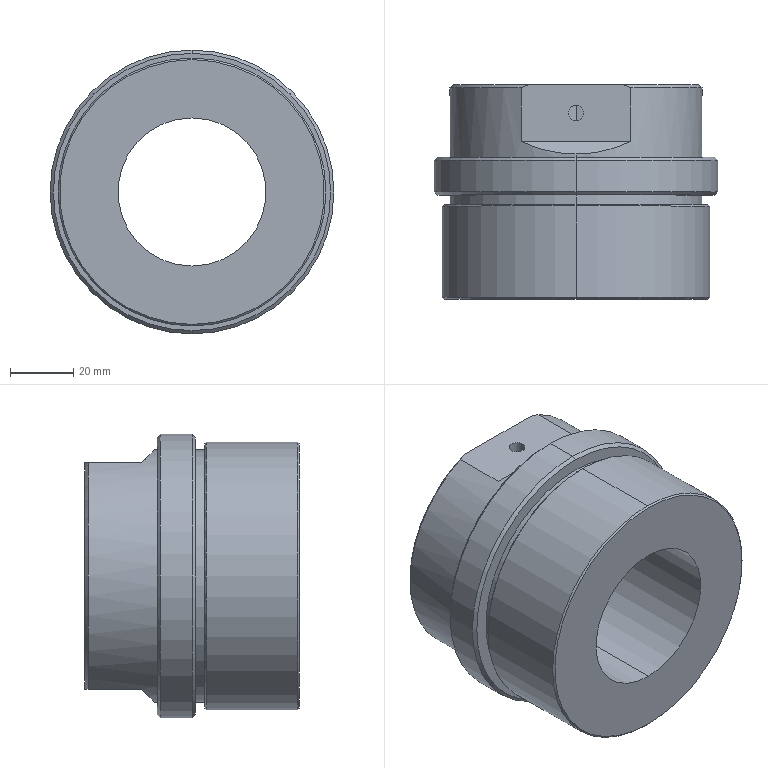Part | SolidWorks | features ICE 14, Chamfer 4, HoleWzd 2, Extrusion 1 | 1 solid | 31 faces | box 90 x 68 x 90 mm | volume 254922 mm3 | cylinder 12 | cone 10 | plane 9 | commonest cylinder face diameters 80 x4 5 x2 47 x2 85 x2 90 x2
STEP:
#1=CARTESIAN_POINT('',(-2.5,21.,23.367));
#2=VERTEX_POINT('',#1);
#3=CARTESIAN_POINT('',(0.,18.5,23.5));
#4=VERTEX_POINT('',#3);
#5=CARTESIAN_POINT('',(-2.5,21.,23.367));
#6=CARTESIAN_POINT('',(-2.5,20.835,23.367));
#7=CARTESIAN_POINT('',(-2.484,20.672,23.368));
#8=CARTESIAN_POINT('',(-2.42,20.353,23.375));
#9=CARTESIAN_POINT('',(-2.372,20.194,23.38));
#10=CARTESIAN_POINT('',(-2.247,19.892,23.392));
#11=CARTESIAN_POINT('',(-2.17,19.748,23.4));
#12=CARTESIAN_POINT('',(-1.989,19.477,23.416));
#13=CARTESIAN_POINT('',(-1.883,19.348,23.425));
#14=CARTESIAN_POINT('',(-1.653,19.118,23.442));
#15=CARTESIAN_POINT('',(-1.528,19.014,23.451));
#16=CARTESIAN_POINT('',(-1.255,18.831,23.467));
#17=CARTESIAN_POINT('',(-1.109,18.754,23.474));
#18=CARTESIAN_POINT('',(-0.6586,18.566,23.493));
#19=CARTESIAN_POINT('',(-0.3304,18.5,23.5));
#20=CARTESIAN_POINT('',(0.,18.5,23.5));
#21=B_SPLINE_CURVE_WITH_KNOTS('',3,(#5,#6,#7,#8,#9,#10,#11,#12,#13,#14,#15,#16,#17,#18,#19,#20),.UNSPECIFIED.,.F.,.F.,(4,2,2,2,2,2,2,4),(0.01173,0.01222,0.01271,0.0132,0.01369,0.01418,0.01466,0.01564),.UNSPECIFIED.);
#22=EDGE_CURVE('',#2,#4,#21,.T.);
#23=ORIENTED_EDGE('',*,*,#22,.F.);
#24=CARTESIAN_POINT('',(-2.5,21.,36.));
#25=VERTEX_POINT('',#24);
#26=CARTESIAN_POINT('',(-2.5,21.,36.));
#27=DIRECTION('',(0.,0.,1.));
#28=VECTOR('',#27,1000.);
#29=LINE('',#26,#28);
#30=EDGE_CURVE('',#2,#25,#29,.T.);
#31=ORIENTED_EDGE('',*,*,#30,.T.);
#32=CARTESIAN_POINT('',(2.5,21.,36.));
#33=VERTEX_POINT('',#32);
#34=CARTESIAN_POINT('',(0.,21.,36.));
#35=DIRECTION('',(0.,0.,1.));
#36=DIRECTION('',(1.,0.,0.));
#37=AXIS2_PLACEMENT_3D('',#34,#35,#36);
#38=CIRCLE('',#37,2.5);
#39=EDGE_CURVE('',#25,#33,#38,.T.);
#40=ORIENTED_EDGE('',*,*,#39,.T.);
#41=CARTESIAN_POINT('',(2.5,21.,23.367));
#42=VERTEX_POINT('',#41);
#43=CARTESIAN_POINT('',(2.5,21.,36.));
#44=DIRECTION('',(0.,0.,1.));
#45=VECTOR('',#44,1000.);
#46=LINE('',#43,#45);
#47=EDGE_CURVE('',#42,#33,#46,.T.);
#48=ORIENTED_EDGE('',*,*,#47,.F.);
#49=CARTESIAN_POINT('',(0.,18.5,23.5));
#50=CARTESIAN_POINT('',(0.1653,18.5,23.5));
#51=CARTESIAN_POINT('',(0.3279,18.516,23.498));
#52=CARTESIAN_POINT('',(0.6477,18.58,23.492));
#53=CARTESIAN_POINT('',(0.8066,18.628,23.487));
#54=CARTESIAN_POINT('',(1.109,18.754,23.474));
#55=CARTESIAN_POINT('',(1.253,18.83,23.467));
#56=CARTESIAN_POINT('',(1.525,19.012,23.451));
#57=CARTESIAN_POINT('',(1.653,19.118,23.442));
#58=CARTESIAN_POINT('',(1.884,19.348,23.425));
#59=CARTESIAN_POINT('',(1.987,19.474,23.416));
#60=CARTESIAN_POINT('',(2.17,19.747,23.4));
#61=CARTESIAN_POINT('',(2.247,19.893,23.392));
#62=CARTESIAN_POINT('',(2.372,20.194,23.38));
#63=CARTESIAN_POINT('',(2.42,20.352,23.375));
#64=CARTESIAN_POINT('',(2.484,20.674,23.368));
#65=CARTESIAN_POINT('',(2.5,20.837,23.367));
#66=CARTESIAN_POINT('',(2.5,21.,23.367));
#67=B_SPLINE_CURVE_WITH_KNOTS('',3,(#49,#50,#51,#52,#53,#54,#55,#56,#57,#58,#59,#60,#61,#62,#63,#64,#65,#66),.UNSPECIFIED.,.F.,.F.,(4,2,2,2,2,2,2,2,4),(0.,0.000489,0.0009779,0.001467,0.001956,0.002445,0.002934,0.003423,0.003912),.UNSPECIFIED.);
#68=EDGE_CURVE('',#4,#42,#67,.T.);
#69=ORIENTED_EDGE('',*,*,#68,.F.);
#70=EDGE_LOOP('',(#23,#31,#40,#48,#69));
#71=FACE_OUTER_BOUND('',#70,.T.);
#72=CARTESIAN_POINT('',(0.,21.,36.));
#73=DIRECTION('',(0.,0.,1.));
#74=DIRECTION('',(1.,0.,0.));
#75=AXIS2_PLACEMENT_3D('',#72,#73,#74);
#76=CYLINDRICAL_SURFACE('',#75,2.5);
#77=ADVANCED_FACE('',(#71),#76,.F.);
#78=CARTESIAN_POINT('',(0.,-8.,42.));
#79=VERTEX_POINT('',#78);
#80=CARTESIAN_POINT('',(0.,-8.,-42.));
#81=VERTEX_POINT('',#80);
#82=CARTESIAN_POINT('',(0.,-8.,0.));
#83=DIRECTION('',(0.,1.,0.));
#84=DIRECTION('',(0.,0.,-1.));
#85=AXIS2_PLACEMENT_3D('',#82,#83,#84);
#86=CIRCLE('',#85,42.);
#87=EDGE_CURVE('',#79,#81,#86,.T.);
#88=ORIENTED_EDGE('',*,*,#87,.F.);
#89=CARTESIAN_POINT('',(0.,-8.5,42.5));
#90=VERTEX_POINT('',#89);
#91=CARTESIAN_POINT('',(0.,-8.5,42.5));
#92=DIRECTION('',(0.,-0.7071,0.7071));
#93=VECTOR('',#92,1000.);
#94=LINE('',#91,#93);
#95=EDGE_CURVE('',#79,#90,#94,.T.);
#96=ORIENTED_EDGE('',*,*,#95,.T.);
#97=CARTESIAN_POINT('',(0.,-8.5,-42.5));
#98=VERTEX_POINT('',#97);
#99=CARTESIAN_POINT('',(0.,-8.5,0.));
#100=DIRECTION('',(0.,-1.,0.));
#101=DIRECTION('',(0.,0.,-1.));
#102=AXIS2_PLACEMENT_3D('',#99,#100,#101);
#103=CIRCLE('',#102,42.5);
#104=EDGE_CURVE('',#98,#90,#103,.T.);
#105=ORIENTED_EDGE('',*,*,#104,.F.);
#106=CARTESIAN_POINT('',(0.,-8.5,-42.5));
#107=DIRECTION('',(0.,-0.7071,-0.7071));
#108=VECTOR('',#107,1000.);
#109=LINE('',#106,#108);
#110=EDGE_CURVE('',#81,#98,#109,.T.);
#111=ORIENTED_EDGE('',*,*,#110,.F.);
#112=EDGE_LOOP('',(#88,#96,#105,#111));
#113=FACE_OUTER_BOUND('',#112,.T.);
#114=CARTESIAN_POINT('',(0.,-8.5,0.));
#115=DIRECTION('',(0.,-1.,0.));
#116=DIRECTION('',(0.,0.,-1.));
#117=AXIS2_PLACEMENT_3D('',#114,#115,#116);
#118=CONICAL_SURFACE('',#117,42.5,0.7854);
#119=ADVANCED_FACE('',(#113),#118,.T.);
#120=CARTESIAN_POINT('',(0.,-38.,-42.));
#121=VERTEX_POINT('',#120);
#122=CARTESIAN_POINT('',(0.,-38.,42.));
#123=VERTEX_POINT('',#122);
#124=CARTESIAN_POINT('',(0.,-38.,0.));
#125=DIRECTION('',(0.,-1.,0.));
#126=DIRECTION('',(0.,0.,-1.));
#127=AXIS2_PLACEMENT_3D('',#124,#125,#126);
#128=CIRCLE('',#127,42.);
#129=EDGE_CURVE('',#121,#123,#128,.T.);
#130=ORIENTED_EDGE('',*,*,#129,.F.);
#131=CARTESIAN_POINT('',(0.,-37.5,-42.5));
#132=VERTEX_POINT('',#131);
#133=CARTESIAN_POINT('',(0.,-38.,-42.));
#134=DIRECTION('',(0.,0.7071,-0.7071));
#135=VECTOR('',#134,1000.);
#136=LINE('',#133,#135);
#137=EDGE_CURVE('',#121,#132,#136,.T.);
#138=ORIENTED_EDGE('',*,*,#137,.T.);
#139=CARTESIAN_POINT('',(0.,-37.5,42.5));
#140=VERTEX_POINT('',#139);
#141=CARTESIAN_POINT('',(0.,-37.5,0.));
#142=DIRECTION('',(0.,1.,0.));
#143=DIRECTION('',(0.,0.,-1.));
#144=AXIS2_PLACEMENT_3D('',#141,#142,#143);
#145=CIRCLE('',#144,42.5);
#146=EDGE_CURVE('',#140,#132,#145,.T.);
#147=ORIENTED_EDGE('',*,*,#146,.F.);
#148=CARTESIAN_POINT('',(0.,-38.,42.));
#149=DIRECTION('',(0.,0.7071,0.7071));
#150=VECTOR('',#149,1000.);
#151=LINE('',#148,#150);
#152=EDGE_CURVE('',#123,#140,#151,.T.);
#153=ORIENTED_EDGE('',*,*,#152,.F.);
#154=EDGE_LOOP('',(#130,#138,#147,#153));
#155=FACE_OUTER_BOUND('',#154,.T.);
#156=CARTESIAN_POINT('',(0.,-38.,0.));
#157=DIRECTION('',(0.,1.,0.));
#158=DIRECTION('',(0.,0.,1.));
#159=AXIS2_PLACEMENT_3D('',#156,#157,#158);
#160=CONICAL_SURFACE('',#159,42.,0.7854);
#161=ADVANCED_FACE('',(#155),#160,.T.);
#162=CARTESIAN_POINT('',(0.,-8.,-40.));
#163=VERTEX_POINT('',#162);
#164=CARTESIAN_POINT('',(0.,-8.,40.));
#165=VERTEX_POINT('',#164);
#166=CARTESIAN_POINT('',(0.,-8.,0.));
#167=DIRECTION('',(0.,-1.,0.));
#168=DIRECTION('',(0.,0.,-1.));
#169=AXIS2_PLACEMENT_3D('',#166,#167,#168);
#170=CIRCLE('',#169,40.);
#171=EDGE_CURVE('',#163,#165,#170,.T.);
#172=ORIENTED_EDGE('',*,*,#171,.F.);
#173=CARTESIAN_POINT('',(0.,-5.,-40.));
#174=VERTEX_POINT('',#173);
#175=CARTESIAN_POINT('',(0.,-8.,-40.));
#176=DIRECTION('',(0.,1.,0.));
#177=VECTOR('',#176,1000.);
#178=LINE('',#175,#177);
#179=EDGE_CURVE('',#163,#174,#178,.T.);
#180=ORIENTED_EDGE('',*,*,#179,.T.);
#181=CARTESIAN_POINT('',(0.,-5.,40.));
#182=VERTEX_POINT('',#181);
#183=CARTESIAN_POINT('',(0.,-5.,0.));
#184=DIRECTION('',(0.,-1.,0.));
#185=DIRECTION('',(0.,0.,-1.));
#186=AXIS2_PLACEMENT_3D('',#183,#184,#185);
#187=CIRCLE('',#186,40.);
#188=EDGE_CURVE('',#174,#182,#187,.T.);
#189=ORIENTED_EDGE('',*,*,#188,.T.);
#190=CARTESIAN_POINT('',(0.,-8.,40.));
#191=DIRECTION('',(0.,1.,0.));
#192=VECTOR('',#191,1000.);
#193=LINE('',#190,#192);
#194=EDGE_CURVE('',#165,#182,#193,.T.);
#195=ORIENTED_EDGE('',*,*,#194,.F.);
#196=EDGE_LOOP('',(#172,#180,#189,#195));
#197=FACE_OUTER_BOUND('',#196,.T.);
#198=CARTESIAN_POINT('',(0.,-8.,0.));
#199=DIRECTION('',(0.,1.,0.));
#200=DIRECTION('',(0.,0.,1.));
#201=AXIS2_PLACEMENT_3D('',#198,#199,#200);
#202=CYLINDRICAL_SURFACE('',#201,40.);
#203=ADVANCED_FACE('',(#197),#202,.T.);
#204=ORIENTED_EDGE('',*,*,#146,.T.);
#205=CARTESIAN_POINT('',(0.,-38.,-42.5));
#206=DIRECTION('',(0.,1.,0.));
#207=VECTOR('',#206,1000.);
#208=LINE('',#205,#207);
#209=EDGE_CURVE('',#132,#98,#208,.T.);
#210=ORIENTED_EDGE('',*,*,#209,.T.);
#211=ORIENTED_EDGE('',*,*,#104,.T.);
#212=CARTESIAN_POINT('',(0.,-38.,42.5));
#213=DIRECTION('',(0.,1.,0.));
#214=VECTOR('',#213,1000.);
#215=LINE('',#212,#214);
#216=EDGE_CURVE('',#140,#90,#215,.T.);
#217=ORIENTED_EDGE('',*,*,#216,.F.);
#218=EDGE_LOOP('',(#204,#210,#211,#217));
#219=FACE_OUTER_BOUND('',#218,.T.);
#220=CARTESIAN_POINT('',(0.,-38.,0.));
#221=DIRECTION('',(0.,1.,0.));
#222=DIRECTION('',(0.,0.,1.));
#223=AXIS2_PLACEMENT_3D('',#220,#221,#222);
#224=CYLINDRICAL_SURFACE('',#223,42.5);
#225=ADVANCED_FACE('',(#219),#224,.T.);
#226=CARTESIAN_POINT('',(0.,-38.,-23.5));
#227=VERTEX_POINT('',#226);
#228=CARTESIAN_POINT('',(0.,-38.,23.5));
#229=VERTEX_POINT('',#228);
#230=CARTESIAN_POINT('',(0.,-38.,0.));
#231=DIRECTION('',(0.,1.,0.));
#232=DIRECTION('',(0.,0.,1.));
#233=AXIS2_PLACEMENT_3D('',#230,#231,#232);
#234=CIRCLE('',#233,23.5);
#235=EDGE_CURVE('',#227,#229,#234,.T.);
#236=ORIENTED_EDGE('',*,*,#235,.F.);
#237=CARTESIAN_POINT('',(0.,30.,-23.5));
#238=VERTEX_POINT('',#237);
#239=CARTESIAN_POINT('',(0.,30.,-23.5));
#240=DIRECTION('',(0.,1.,0.));
#241=VECTOR('',#240,1000.);
#242=LINE('',#239,#241);
#243=EDGE_CURVE('',#227,#238,#242,.T.);
#244=ORIENTED_EDGE('',*,*,#243,.T.);
#245=CARTESIAN_POINT('',(0.,30.,23.5));
#246=VERTEX_POINT('',#245);
#247=CARTESIAN_POINT('',(0.,30.,0.));
#248=DIRECTION('',(0.,1.,0.));
#249=DIRECTION('',(0.,0.,1.));
#250=AXIS2_PLACEMENT_3D('',#247,#248,#249);
#251=CIRCLE('',#250,23.5);
#252=EDGE_CURVE('',#238,#246,#251,.T.);
#253=ORIENTED_EDGE('',*,*,#252,.T.);
#254=CARTESIAN_POINT('',(0.,23.5,23.5));
#255=VERTEX_POINT('',#254);
#256=CARTESIAN_POINT('',(0.,30.,23.5));
#257=DIRECTION('',(0.,1.,0.));
#258=VECTOR('',#257,1000.);
#259=LINE('',#256,#258);
#260=EDGE_CURVE('',#255,#246,#259,.T.);
#261=ORIENTED_EDGE('',*,*,#260,.F.);
#262=CARTESIAN_POINT('',(0.,23.5,23.5));
#263=CARTESIAN_POINT('',(-0.1633,23.5,23.5));
#264=CARTESIAN_POINT('',(-0.3256,23.484,23.498));
#265=CARTESIAN_POINT('',(-0.6484,23.42,23.492));
#266=CARTESIAN_POINT('',(-0.8062,23.372,23.487));
#267=CARTESIAN_POINT('',(-1.107,23.247,23.474));
#268=CARTESIAN_POINT('',(-1.253,23.17,23.467));
#269=CARTESIAN_POINT('',(-1.526,22.987,23.451));
#270=CARTESIAN_POINT('',(-1.652,22.884,23.442));
#271=CARTESIAN_POINT('',(-1.883,22.653,23.425));
#272=CARTESIAN_POINT('',(-1.988,22.524,23.416));
#273=CARTESIAN_POINT('',(-2.17,22.253,23.4));
#274=CARTESIAN_POINT('',(-2.246,22.109,23.392));
#275=CARTESIAN_POINT('',(-2.372,21.806,23.38));
#276=CARTESIAN_POINT('',(-2.42,21.648,23.375));
#277=CARTESIAN_POINT('',(-2.484,21.328,23.368));
#278=CARTESIAN_POINT('',(-2.5,21.165,23.367));
#279=CARTESIAN_POINT('',(-2.5,21.,23.367));
#280=B_SPLINE_CURVE_WITH_KNOTS('',3,(#262,#263,#264,#265,#266,#267,#268,#269,#270,#271,#272,#273,#274,#275,#276,#277,#278,#279),.UNSPECIFIED.,.F.,.F.,(4,2,2,2,2,2,2,2,4),(0.007822,0.008311,0.0088,0.009289,0.009778,0.01027,0.01076,0.01124,0.01173),.UNSPECIFIED.);
#281=EDGE_CURVE('',#255,#2,#280,.T.);
#282=ORIENTED_EDGE('',*,*,#281,.T.);
#283=ORIENTED_EDGE('',*,*,#22,.T.);
#284=CARTESIAN_POINT('',(0.,30.,23.5));
#285=DIRECTION('',(0.,1.,0.));
#286=VECTOR('',#285,1000.);
#287=LINE('',#284,#286);
#288=EDGE_CURVE('',#229,#4,#287,.T.);
#289=ORIENTED_EDGE('',*,*,#288,.F.);
#290=EDGE_LOOP('',(#236,#244,#253,#261,#282,#283,#289));
#291=FACE_OUTER_BOUND('',#290,.T.);
#292=CARTESIAN_POINT('',(0.,30.,0.));
#293=DIRECTION('',(0.,1.,0.));
#294=DIRECTION('',(0.,0.,1.));
#295=AXIS2_PLACEMENT_3D('',#292,#293,#294);
#296=CYLINDRICAL_SURFACE('',#295,23.5);
#297=ADVANCED_FACE('',(#291),#296,.F.);
#298=CARTESIAN_POINT('',(0.,7.,44.));
#299=VERTEX_POINT('',#298);
#300=CARTESIAN_POINT('',(0.,7.,-44.));
#301=VERTEX_POINT('',#300);
#302=CARTESIAN_POINT('',(0.,7.,0.));
#303=DIRECTION('',(0.,1.,0.));
#304=DIRECTION('',(0.,0.,1.));
#305=AXIS2_PLACEMENT_3D('',#302,#303,#304);
#306=CIRCLE('',#305,44.);
#307=EDGE_CURVE('',#299,#301,#306,.T.);
#308=ORIENTED_EDGE('',*,*,#307,.F.);
#309=CARTESIAN_POINT('',(0.,6.,45.));
#310=VERTEX_POINT('',#309);
#311=CARTESIAN_POINT('',(0.,7.,44.));
#312=DIRECTION('',(0.,-0.7071,0.7071));
#313=VECTOR('',#312,1000.);
#314=LINE('',#311,#313);
#315=EDGE_CURVE('',#299,#310,#314,.T.);
#316=ORIENTED_EDGE('',*,*,#315,.T.);
#317=CARTESIAN_POINT('',(0.,6.,-45.));
#318=VERTEX_POINT('',#317);
#319=CARTESIAN_POINT('',(0.,6.,0.));
#320=DIRECTION('',(0.,-1.,0.));
#321=DIRECTION('',(0.,0.,1.));
#322=AXIS2_PLACEMENT_3D('',#319,#320,#321);
#323=CIRCLE('',#322,45.);
#324=EDGE_CURVE('',#318,#310,#323,.T.);
#325=ORIENTED_EDGE('',*,*,#324,.F.);
#326=CARTESIAN_POINT('',(0.,7.,-44.));
#327=DIRECTION('',(0.,-0.7071,-0.7071));
#328=VECTOR('',#327,1000.);
#329=LINE('',#326,#328);
#330=EDGE_CURVE('',#301,#318,#329,.T.);
#331=ORIENTED_EDGE('',*,*,#330,.F.);
#332=EDGE_LOOP('',(#308,#316,#325,#331));
#333=FACE_OUTER_BOUND('',#332,.T.);
#334=CARTESIAN_POINT('',(0.,7.,0.));
#335=DIRECTION('',(0.,-1.,0.));
#336=DIRECTION('',(0.,0.,-1.));
#337=AXIS2_PLACEMENT_3D('',#334,#335,#336);
#338=CONICAL_SURFACE('',#337,44.,0.7854);
#339=ADVANCED_FACE('',(#333),#338,.T.);
#340=ORIENTED_EDGE('',*,*,#324,.T.);
#341=CARTESIAN_POINT('',(0.,-4.,45.));
#342=VERTEX_POINT('',#341);
#343=CARTESIAN_POINT('',(0.,5.,45.));
#344=DIRECTION('',(0.,-1.,0.));
#345=VECTOR('',#344,1000.);
#346=LINE('',#343,#345);
#347=EDGE_CURVE('',#310,#342,#346,.T.);
#348=ORIENTED_EDGE('',*,*,#347,.T.);
#349=CARTESIAN_POINT('',(0.,-4.,-45.));
#350=VERTEX_POINT('',#349);
#351=CARTESIAN_POINT('',(0.,-4.,0.));
#352=DIRECTION('',(0.,1.,0.));
#353=DIRECTION('',(0.,0.,-1.));
#354=AXIS2_PLACEMENT_3D('',#351,#352,#353);
#355=CIRCLE('',#354,45.);
#356=EDGE_CURVE('',#342,#350,#355,.T.);
#357=ORIENTED_EDGE('',*,*,#356,.T.);
#358=CARTESIAN_POINT('',(0.,5.,-45.));
#359=DIRECTION('',(0.,-1.,0.));
#360=VECTOR('',#359,1000.);
#361=LINE('',#358,#360);
#362=EDGE_CURVE('',#318,#350,#361,.T.);
#363=ORIENTED_EDGE('',*,*,#362,.F.);
#364=EDGE_LOOP('',(#340,#348,#357,#363));
#365=FACE_OUTER_BOUND('',#364,.T.);
#366=CARTESIAN_POINT('',(0.,5.,0.));
#367=DIRECTION('',(0.,-1.,0.));
#368=DIRECTION('',(0.,0.,-1.));
#369=AXIS2_PLACEMENT_3D('',#366,#367,#368);
#370=CYLINDRICAL_SURFACE('',#369,45.);
#371=ADVANCED_FACE('',(#365),#370,.T.);
#372=CARTESIAN_POINT('',(0.,-5.,-44.));
#373=VERTEX_POINT('',#372);
#374=CARTESIAN_POINT('',(0.,-5.,44.));
#375=VERTEX_POINT('',#374);
#376=CARTESIAN_POINT('',(0.,-5.,0.));
#377=DIRECTION('',(0.,-1.,0.));
#378=DIRECTION('',(0.,0.,-1.));
#379=AXIS2_PLACEMENT_3D('',#376,#377,#378);
#380=CIRCLE('',#379,44.);
#381=EDGE_CURVE('',#373,#375,#380,.T.);
#382=ORIENTED_EDGE('',*,*,#381,.F.);
#383=CARTESIAN_POINT('',(0.,-5.,-44.));
#384=DIRECTION('',(0.,0.7071,-0.7071));
#385=VECTOR('',#384,1000.);
#386=LINE('',#383,#385);
#387=EDGE_CURVE('',#373,#350,#386,.T.);
#388=ORIENTED_EDGE('',*,*,#387,.T.);
#389=ORIENTED_EDGE('',*,*,#356,.F.);
#390=CARTESIAN_POINT('',(0.,-5.,44.));
#391=DIRECTION('',(0.,0.7071,0.7071));
#392=VECTOR('',#391,1000.);
#393=LINE('',#390,#392);
#394=EDGE_CURVE('',#375,#342,#393,.T.);
#395=ORIENTED_EDGE('',*,*,#394,.F.);
#396=EDGE_LOOP('',(#382,#388,#389,#395));
#397=FACE_OUTER_BOUND('',#396,.T.);
#398=CARTESIAN_POINT('',(0.,-5.,0.));
#399=DIRECTION('',(0.,1.,0.));
#400=DIRECTION('',(0.,0.,1.));
#401=AXIS2_PLACEMENT_3D('',#398,#399,#400);
#402=CONICAL_SURFACE('',#401,44.,0.7854);
#403=ADVANCED_FACE('',(#397),#402,.T.);
#404=CARTESIAN_POINT('',(17.436,12.,36.));
#405=VERTEX_POINT('',#404);
#406=CARTESIAN_POINT('',(0.,8.,40.));
#407=VERTEX_POINT('',#406);
#408=CARTESIAN_POINT('',(17.436,12.,36.));
#409=CARTESIAN_POINT('',(11.977,9.356,38.644));
#410=CARTESIAN_POINT('',(6.065,8.,40.));
#411=CARTESIAN_POINT('',(0.,8.,40.));
#412=(BOUNDED_CURVE()B_SPLINE_CURVE(3,(#408,#409,#410,#411),.UNSPECIFIED.,.F.,.F.)B_SPLINE_CURVE_WITH_KNOTS((4,4),(5.832,6.283),.UNSPECIFIED.)CURVE()GEOMETRIC_REPRESENTATION_ITEM()RATIONAL_B_SPLINE_CURVE((1.,0.9831,0.9831,1.))REPRESENTATION_ITEM(''));
#413=EDGE_CURVE('',#405,#407,#412,.T.);
#414=ORIENTED_EDGE('',*,*,#413,.T.);
#415=CARTESIAN_POINT('',(0.,7.,40.));
#416=VERTEX_POINT('',#415);
#417=CARTESIAN_POINT('',(0.,30.,40.));
#418=DIRECTION('',(0.,-1.,0.));
#419=VECTOR('',#418,1000.);
#420=LINE('',#417,#419);
#421=EDGE_CURVE('',#407,#416,#420,.T.);
#422=ORIENTED_EDGE('',*,*,#421,.T.);
#423=CARTESIAN_POINT('',(0.,7.,-40.));
#424=VERTEX_POINT('',#423);
#425=CARTESIAN_POINT('',(0.,7.,0.));
#426=DIRECTION('',(0.,1.,0.));
#427=DIRECTION('',(0.,0.,1.));
#428=AXIS2_PLACEMENT_3D('',#425,#426,#427);
#429=CIRCLE('',#428,40.);
#430=EDGE_CURVE('',#416,#424,#429,.T.);
#431=ORIENTED_EDGE('',*,*,#430,.T.);
#432=CARTESIAN_POINT('',(0.,8.,-40.));
#433=VERTEX_POINT('',#432);
#434=CARTESIAN_POINT('',(0.,30.,-40.));
#435=DIRECTION('',(0.,-1.,0.));
#436=VECTOR('',#435,1000.);
#437=LINE('',#434,#436);
#438=EDGE_CURVE('',#433,#424,#437,.T.);
#439=ORIENTED_EDGE('',*,*,#438,.F.);
#440=CARTESIAN_POINT('',(17.436,12.,-36.));
#441=VERTEX_POINT('',#440);
#442=CARTESIAN_POINT('',(0.,8.,-40.));
#443=CARTESIAN_POINT('',(6.065,8.,-40.));
#444=CARTESIAN_POINT('',(11.977,9.356,-38.644));
#445=CARTESIAN_POINT('',(17.436,12.,-36.));
#446=(BOUNDED_CURVE()B_SPLINE_CURVE(3,(#442,#443,#444,#445),.UNSPECIFIED.,.F.,.F.)B_SPLINE_CURVE_WITH_KNOTS((4,4),(0.,0.451),.UNSPECIFIED.)CURVE()GEOMETRIC_REPRESENTATION_ITEM()RATIONAL_B_SPLINE_CURVE((1.,0.9831,0.9831,1.))REPRESENTATION_ITEM(''));
#447=EDGE_CURVE('',#433,#441,#446,.T.);
#448=ORIENTED_EDGE('',*,*,#447,.T.);
#449=CARTESIAN_POINT('',(17.436,29.,-36.));
#450=VERTEX_POINT('',#449);
#451=CARTESIAN_POINT('',(17.436,30.,-36.));
#452=DIRECTION('',(0.,1.,0.));
#453=VECTOR('',#452,1000.);
#454=LINE('',#451,#453);
#455=EDGE_CURVE('',#441,#450,#454,.T.);
#456=ORIENTED_EDGE('',*,*,#455,.T.);
#457=CARTESIAN_POINT('',(17.436,29.,36.));
#458=VERTEX_POINT('',#457);
#459=CARTESIAN_POINT('',(0.,29.,0.));
#460=DIRECTION('',(0.,-1.,0.));
#461=DIRECTION('',(0.,0.,1.));
#462=AXIS2_PLACEMENT_3D('',#459,#460,#461);
#463=CIRCLE('',#462,40.);
#464=EDGE_CURVE('',#450,#458,#463,.T.);
#465=ORIENTED_EDGE('',*,*,#464,.T.);
#466=CARTESIAN_POINT('',(17.436,30.,36.));
#467=DIRECTION('',(0.,-1.,0.));
#468=VECTOR('',#467,1000.);
#469=LINE('',#466,#468);
#470=EDGE_CURVE('',#458,#405,#469,.T.);
#471=ORIENTED_EDGE('',*,*,#470,.T.);
#472=EDGE_LOOP('',(#414,#422,#431,#439,#448,#456,#465,#471));
#473=FACE_OUTER_BOUND('',#472,.T.);
#474=CARTESIAN_POINT('',(0.,30.,0.));
#475=DIRECTION('',(0.,-1.,0.));
#476=DIRECTION('',(0.,0.,-1.));
#477=AXIS2_PLACEMENT_3D('',#474,#475,#476);
#478=CYLINDRICAL_SURFACE('',#477,40.);
#479=ADVANCED_FACE('',(#473),#478,.T.);
#480=ORIENTED_EDGE('',*,*,#470,.F.);
#481=CARTESIAN_POINT('',(15.,30.,36.));
#482=VERTEX_POINT('',#481);
#483=CARTESIAN_POINT('',(17.436,29.,36.));
#484=CARTESIAN_POINT('',(16.631,29.351,36.));
#485=CARTESIAN_POINT('',(15.819,29.685,36.));
#486=CARTESIAN_POINT('',(15.,30.,36.));
#487=B_SPLINE_CURVE_WITH_KNOTS('',3,(#483,#484,#485,#486),.UNSPECIFIED.,.F.,.F.,(4,4),(0.,0.002633),.UNSPECIFIED.);
#488=EDGE_CURVE('',#458,#482,#487,.T.);
#489=ORIENTED_EDGE('',*,*,#488,.T.);
#490=CARTESIAN_POINT('',(-15.,30.,36.));
#491=VERTEX_POINT('',#490);
#492=CARTESIAN_POINT('',(-41.342,30.,36.));
#493=DIRECTION('',(-1.,0.,0.));
#494=VECTOR('',#493,1000.);
#495=LINE('',#492,#494);
#496=EDGE_CURVE('',#482,#491,#495,.T.);
#497=ORIENTED_EDGE('',*,*,#496,.T.);
#498=CARTESIAN_POINT('',(-17.436,29.,36.));
#499=VERTEX_POINT('',#498);
#500=CARTESIAN_POINT('',(-15.,30.,36.));
#501=CARTESIAN_POINT('',(-15.819,29.685,36.));
#502=CARTESIAN_POINT('',(-16.631,29.351,36.));
#503=CARTESIAN_POINT('',(-17.436,29.,36.));
#504=B_SPLINE_CURVE_WITH_KNOTS('',3,(#500,#501,#502,#503),.UNSPECIFIED.,.F.,.F.,(4,4),(0.,0.002633),.UNSPECIFIED.);
#505=EDGE_CURVE('',#491,#499,#504,.T.);
#506=ORIENTED_EDGE('',*,*,#505,.T.);
#507=CARTESIAN_POINT('',(-17.436,12.,36.));
#508=VERTEX_POINT('',#507);
#509=CARTESIAN_POINT('',(-17.436,30.,36.));
#510=DIRECTION('',(0.,1.,0.));
#511=VECTOR('',#510,1000.);
#512=LINE('',#509,#511);
#513=EDGE_CURVE('',#508,#499,#512,.T.);
#514=ORIENTED_EDGE('',*,*,#513,.F.);
#515=CARTESIAN_POINT('',(-41.342,12.,36.));
#516=DIRECTION('',(-1.,0.,0.));
#517=VECTOR('',#516,1000.);
#518=LINE('',#515,#517);
#519=EDGE_CURVE('',#405,#508,#518,.T.);
#520=ORIENTED_EDGE('',*,*,#519,.F.);
#521=EDGE_LOOP('',(#480,#489,#497,#506,#514,#520));
#522=FACE_OUTER_BOUND('',#521,.T.);
#523=CARTESIAN_POINT('',(0.,21.,36.));
#524=DIRECTION('',(0.,0.,1.));
#525=DIRECTION('',(1.,0.,0.));
#526=AXIS2_PLACEMENT_3D('',#523,#524,#525);
#527=CIRCLE('',#526,2.5);
#528=EDGE_CURVE('',#33,#25,#527,.T.);
#529=ORIENTED_EDGE('',*,*,#528,.F.);
#530=ORIENTED_EDGE('',*,*,#39,.F.);
#531=EDGE_LOOP('',(#529,#530));
#532=FACE_BOUND('',#531,.T.);
#533=CARTESIAN_POINT('',(-41.342,12.,36.));
#534=DIRECTION('',(0.,0.,-1.));
#535=DIRECTION('',(-1.,0.,0.));
#536=AXIS2_PLACEMENT_3D('',#533,#534,#535);
#537=PLANE('',#536);
#538=ADVANCED_FACE('',(#522,#532),#537,.F.);
#539=CARTESIAN_POINT('',(-15.,30.,-36.));
#540=VERTEX_POINT('',#539);
#541=CARTESIAN_POINT('',(15.,30.,-36.));
#542=VERTEX_POINT('',#541);
#543=CARTESIAN_POINT('',(-41.342,30.,-36.));
#544=DIRECTION('',(1.,0.,0.));
#545=VECTOR('',#544,1000.);
#546=LINE('',#543,#545);
#547=EDGE_CURVE('',#540,#542,#546,.T.);
#548=ORIENTED_EDGE('',*,*,#547,.T.);
#549=CARTESIAN_POINT('',(15.,30.,-36.));
#550=CARTESIAN_POINT('',(15.819,29.685,-36.));
#551=CARTESIAN_POINT('',(16.631,29.351,-36.));
#552=CARTESIAN_POINT('',(17.436,29.,-36.));
#553=B_SPLINE_CURVE_WITH_KNOTS('',3,(#549,#550,#551,#552),.UNSPECIFIED.,.F.,.F.,(4,4),(0.,0.002633),.UNSPECIFIED.);
#554=EDGE_CURVE('',#542,#450,#553,.T.);
#555=ORIENTED_EDGE('',*,*,#554,.T.);
#556=ORIENTED_EDGE('',*,*,#455,.F.);
#557=CARTESIAN_POINT('',(-17.436,12.,-36.));
#558=VERTEX_POINT('',#557);
#559=CARTESIAN_POINT('',(-41.342,12.,-36.));
#560=DIRECTION('',(1.,0.,0.));
#561=VECTOR('',#560,1000.);
#562=LINE('',#559,#561);
#563=EDGE_CURVE('',#558,#441,#562,.T.);
#564=ORIENTED_EDGE('',*,*,#563,.F.);
#565=CARTESIAN_POINT('',(-17.436,29.,-36.));
#566=VERTEX_POINT('',#565);
#567=CARTESIAN_POINT('',(-17.436,30.,-36.));
#568=DIRECTION('',(0.,-1.,0.));
#569=VECTOR('',#568,1000.);
#570=LINE('',#567,#569);
#571=EDGE_CURVE('',#566,#558,#570,.T.);
#572=ORIENTED_EDGE('',*,*,#571,.F.);
#573=CARTESIAN_POINT('',(-17.436,29.,-36.));
#574=CARTESIAN_POINT('',(-16.631,29.351,-36.));
#575=CARTESIAN_POINT('',(-15.819,29.685,-36.));
#576=CARTESIAN_POINT('',(-15.,30.,-36.));
#577=B_SPLINE_CURVE_WITH_KNOTS('',3,(#573,#574,#575,#576),.UNSPECIFIED.,.F.,.F.,(4,4),(0.,0.002633),.UNSPECIFIED.);
#578=EDGE_CURVE('',#566,#540,#577,.T.);
#579=ORIENTED_EDGE('',*,*,#578,.T.);
#580=EDGE_LOOP('',(#548,#555,#556,#564,#572,#579));
#581=FACE_OUTER_BOUND('',#580,.T.);
#582=CARTESIAN_POINT('',(-41.342,12.,-36.));
#583=DIRECTION('',(0.,0.,1.));
#584=DIRECTION('',(1.,0.,0.));
#585=AXIS2_PLACEMENT_3D('',#582,#583,#584);
#586=PLANE('',#585);
#587=ADVANCED_FACE('',(#581),#586,.F.);
#588=CARTESIAN_POINT('',(0.,30.,0.));
#589=DIRECTION('',(0.,1.,0.));
#590=DIRECTION('',(0.,0.,1.));
#591=AXIS2_PLACEMENT_3D('',#588,#589,#590);
#592=CIRCLE('',#591,23.5);
#593=EDGE_CURVE('',#246,#238,#592,.T.);
#594=ORIENTED_EDGE('',*,*,#593,.F.);
#595=ORIENTED_EDGE('',*,*,#252,.F.);
#596=EDGE_LOOP('',(#594,#595));
#597=FACE_BOUND('',#596,.T.);
#598=ORIENTED_EDGE('',*,*,#496,.F.);
#599=CARTESIAN_POINT('',(0.,30.,0.));
#600=DIRECTION('',(0.,1.,0.));
#601=DIRECTION('',(0.,0.,1.));
#602=AXIS2_PLACEMENT_3D('',#599,#600,#601);
#603=CIRCLE('',#602,39.);
#604=EDGE_CURVE('',#482,#542,#603,.T.);
#605=ORIENTED_EDGE('',*,*,#604,.T.);
#606=ORIENTED_EDGE('',*,*,#547,.F.);
#607=CARTESIAN_POINT('',(0.,30.,0.));
#608=DIRECTION('',(0.,1.,0.));
#609=DIRECTION('',(0.,0.,1.));
#610=AXIS2_PLACEMENT_3D('',#607,#608,#609);
#611=CIRCLE('',#610,39.);
#612=EDGE_CURVE('',#540,#491,#611,.T.);
#613=ORIENTED_EDGE('',*,*,#612,.T.);
#614=EDGE_LOOP('',(#598,#605,#606,#613));
#615=FACE_OUTER_BOUND('',#614,.T.);
#616=CARTESIAN_POINT('',(0.,30.,0.));
#617=DIRECTION('',(0.,1.,0.));
#618=DIRECTION('',(0.,0.,1.));
#619=AXIS2_PLACEMENT_3D('',#616,#617,#618);
#620=PLANE('',#619);
#621=ADVANCED_FACE('',(#597,#615),#620,.T.);
#622=ORIENTED_EDGE('',*,*,#421,.F.);
#623=CARTESIAN_POINT('',(0.,8.,40.));
#624=CARTESIAN_POINT('',(-6.065,8.,40.));
#625=CARTESIAN_POINT('',(-11.977,9.356,38.644));
#626=CARTESIAN_POINT('',(-17.436,12.,36.));
#627=(BOUNDED_CURVE()B_SPLINE_CURVE(3,(#623,#624,#625,#626),.UNSPECIFIED.,.F.,.F.)B_SPLINE_CURVE_WITH_KNOTS((4,4),(0.,0.451),.UNSPECIFIED.)CURVE()GEOMETRIC_REPRESENTATION_ITEM()RATIONAL_B_SPLINE_CURVE((1.,0.9831,0.9831,1.))REPRESENTATION_ITEM(''));
#628=EDGE_CURVE('',#407,#508,#627,.T.);
#629=ORIENTED_EDGE('',*,*,#628,.T.);
#630=ORIENTED_EDGE('',*,*,#513,.T.);
#631=CARTESIAN_POINT('',(0.,29.,0.));
#632=DIRECTION('',(0.,-1.,0.));
#633=DIRECTION('',(0.,0.,1.));
#634=AXIS2_PLACEMENT_3D('',#631,#632,#633);
#635=CIRCLE('',#634,40.);
#636=EDGE_CURVE('',#499,#566,#635,.T.);
#637=ORIENTED_EDGE('',*,*,#636,.T.);
#638=ORIENTED_EDGE('',*,*,#571,.T.);
#639=CARTESIAN_POINT('',(-17.436,12.,-36.));
#640=CARTESIAN_POINT('',(-11.977,9.356,-38.644));
#641=CARTESIAN_POINT('',(-6.065,8.,-40.));
#642=CARTESIAN_POINT('',(0.,8.,-40.));
#643=(BOUNDED_CURVE()B_SPLINE_CURVE(3,(#639,#640,#641,#642),.UNSPECIFIED.,.F.,.F.)B_SPLINE_CURVE_WITH_KNOTS((4,4),(5.832,6.283),.UNSPECIFIED.)CURVE()GEOMETRIC_REPRESENTATION_ITEM()RATIONAL_B_SPLINE_CURVE((1.,0.9831,0.9831,1.))REPRESENTATION_ITEM(''));
#644=EDGE_CURVE('',#558,#433,#643,.T.);
#645=ORIENTED_EDGE('',*,*,#644,.T.);
#646=ORIENTED_EDGE('',*,*,#438,.T.);
#647=CARTESIAN_POINT('',(0.,7.,0.));
#648=DIRECTION('',(0.,1.,0.));
#649=DIRECTION('',(0.,0.,1.));
#650=AXIS2_PLACEMENT_3D('',#647,#648,#649);
#651=CIRCLE('',#650,40.);
#652=EDGE_CURVE('',#424,#416,#651,.T.);
#653=ORIENTED_EDGE('',*,*,#652,.T.);
#654=EDGE_LOOP('',(#622,#629,#630,#637,#638,#645,#646,#653));
#655=FACE_OUTER_BOUND('',#654,.T.);
#656=CARTESIAN_POINT('',(0.,30.,0.));
#657=DIRECTION('',(0.,-1.,0.));
#658=DIRECTION('',(0.,0.,-1.));
#659=AXIS2_PLACEMENT_3D('',#656,#657,#658);
#660=CYLINDRICAL_SURFACE('',#659,40.);
#661=ADVANCED_FACE('',(#655),#660,.T.);
#662=ORIENTED_EDGE('',*,*,#488,.F.);
#663=ORIENTED_EDGE('',*,*,#464,.F.);
#664=ORIENTED_EDGE('',*,*,#554,.F.);
#665=ORIENTED_EDGE('',*,*,#604,.F.);
#666=EDGE_LOOP('',(#662,#663,#664,#665));
#667=FACE_OUTER_BOUND('',#666,.T.);
#668=CARTESIAN_POINT('',(0.,30.,0.));
#669=DIRECTION('',(0.,-1.,0.));
#670=DIRECTION('',(0.,0.,-1.));
#671=AXIS2_PLACEMENT_3D('',#668,#669,#670);
#672=CONICAL_SURFACE('',#671,39.,0.7854);
#673=ADVANCED_FACE('',(#667),#672,.T.);
#674=ORIENTED_EDGE('',*,*,#578,.F.);
#675=ORIENTED_EDGE('',*,*,#636,.F.);
#676=ORIENTED_EDGE('',*,*,#505,.F.);
#677=ORIENTED_EDGE('',*,*,#612,.F.);
#678=EDGE_LOOP('',(#674,#675,#676,#677));
#679=FACE_OUTER_BOUND('',#678,.T.);
#680=CARTESIAN_POINT('',(0.,30.,0.));
#681=DIRECTION('',(0.,-1.,0.));
#682=DIRECTION('',(0.,0.,-1.));
#683=AXIS2_PLACEMENT_3D('',#680,#681,#682);
#684=CONICAL_SURFACE('',#683,39.,0.7854);
#685=ADVANCED_FACE('',(#679),#684,.T.);
#686=ORIENTED_EDGE('',*,*,#413,.F.);
#687=ORIENTED_EDGE('',*,*,#519,.T.);
#688=ORIENTED_EDGE('',*,*,#628,.F.);
#689=EDGE_LOOP('',(#686,#687,#688));
#690=FACE_OUTER_BOUND('',#689,.T.);
#691=CARTESIAN_POINT('',(-45.,8.,40.));
#692=DIRECTION('',(0.,-0.7071,-0.7071));
#693=DIRECTION('',(0.,0.7071,-0.7071));
#694=AXIS2_PLACEMENT_3D('',#691,#692,#693);
#695=PLANE('',#694);
#696=ADVANCED_FACE('',(#690),#695,.F.);
#697=ORIENTED_EDGE('',*,*,#563,.T.);
#698=ORIENTED_EDGE('',*,*,#447,.F.);
#699=ORIENTED_EDGE('',*,*,#644,.F.);
#700=EDGE_LOOP('',(#697,#698,#699));
#701=FACE_OUTER_BOUND('',#700,.T.);
#702=CARTESIAN_POINT('',(-45.,6.039,-41.961));
#703=DIRECTION('',(0.,-0.7071,0.7071));
#704=DIRECTION('',(0.,-0.7071,-0.7071));
#705=AXIS2_PLACEMENT_3D('',#702,#703,#704);
#706=PLANE('',#705);
#707=ADVANCED_FACE('',(#701),#706,.F.);
#708=CARTESIAN_POINT('',(0.,7.,0.));
#709=DIRECTION('',(0.,1.,0.));
#710=DIRECTION('',(0.,0.,1.));
#711=AXIS2_PLACEMENT_3D('',#708,#709,#710);
#712=CIRCLE('',#711,44.);
#713=EDGE_CURVE('',#301,#299,#712,.T.);
#714=ORIENTED_EDGE('',*,*,#713,.T.);
#715=ORIENTED_EDGE('',*,*,#307,.T.);
#716=EDGE_LOOP('',(#714,#715));
#717=FACE_OUTER_BOUND('',#716,.T.);
#718=ORIENTED_EDGE('',*,*,#652,.F.);
#719=ORIENTED_EDGE('',*,*,#430,.F.);
#720=EDGE_LOOP('',(#718,#719));
#721=FACE_BOUND('',#720,.T.);
#722=CARTESIAN_POINT('',(0.,7.,0.));
#723=DIRECTION('',(0.,1.,0.));
#724=DIRECTION('',(0.,0.,1.));
#725=AXIS2_PLACEMENT_3D('',#722,#723,#724);
#726=PLANE('',#725);
#727=ADVANCED_FACE('',(#717,#721),#726,.T.);
#728=CARTESIAN_POINT('',(0.,-38.,0.));
#729=DIRECTION('',(0.,-1.,0.));
#730=DIRECTION('',(0.,0.,-1.));
#731=AXIS2_PLACEMENT_3D('',#728,#729,#730);
#732=CIRCLE('',#731,42.);
#733=EDGE_CURVE('',#123,#121,#732,.T.);
#734=ORIENTED_EDGE('',*,*,#733,.T.);
#735=ORIENTED_EDGE('',*,*,#129,.T.);
#736=EDGE_LOOP('',(#734,#735));
#737=FACE_OUTER_BOUND('',#736,.T.);
#738=CARTESIAN_POINT('',(0.,-38.,0.));
#739=DIRECTION('',(0.,1.,0.));
#740=DIRECTION('',(0.,0.,1.));
#741=AXIS2_PLACEMENT_3D('',#738,#739,#740);
#742=CIRCLE('',#741,23.5);
#743=EDGE_CURVE('',#229,#227,#742,.T.);
#744=ORIENTED_EDGE('',*,*,#743,.T.);
#745=ORIENTED_EDGE('',*,*,#235,.T.);
#746=EDGE_LOOP('',(#744,#745));
#747=FACE_BOUND('',#746,.T.);
#748=CARTESIAN_POINT('',(0.,-38.,0.));
#749=DIRECTION('',(0.,-1.,0.));
#750=DIRECTION('',(0.,0.,-1.));
#751=AXIS2_PLACEMENT_3D('',#748,#749,#750);
#752=PLANE('',#751);
#753=ADVANCED_FACE('',(#737,#747),#752,.T.);
#754=CARTESIAN_POINT('',(0.,-5.,0.));
#755=DIRECTION('',(0.,-1.,0.));
#756=DIRECTION('',(0.,0.,-1.));
#757=AXIS2_PLACEMENT_3D('',#754,#755,#756);
#758=CIRCLE('',#757,44.);
#759=EDGE_CURVE('',#375,#373,#758,.T.);
#760=ORIENTED_EDGE('',*,*,#759,.T.);
#761=ORIENTED_EDGE('',*,*,#381,.T.);
#762=EDGE_LOOP('',(#760,#761));
#763=FACE_OUTER_BOUND('',#762,.T.);
#764=CARTESIAN_POINT('',(0.,-5.,0.));
#765=DIRECTION('',(0.,-1.,0.));
#766=DIRECTION('',(0.,0.,-1.));
#767=AXIS2_PLACEMENT_3D('',#764,#765,#766);
#768=CIRCLE('',#767,40.);
#769=EDGE_CURVE('',#182,#174,#768,.T.);
#770=ORIENTED_EDGE('',*,*,#769,.F.);
#771=ORIENTED_EDGE('',*,*,#188,.F.);
#772=EDGE_LOOP('',(#770,#771));
#773=FACE_BOUND('',#772,.T.);
#774=CARTESIAN_POINT('',(0.,-5.,0.));
#775=DIRECTION('',(0.,-1.,0.));
#776=DIRECTION('',(0.,0.,-1.));
#777=AXIS2_PLACEMENT_3D('',#774,#775,#776);
#778=PLANE('',#777);
#779=ADVANCED_FACE('',(#763,#773),#778,.T.);
#780=ORIENTED_EDGE('',*,*,#387,.F.);
#781=ORIENTED_EDGE('',*,*,#759,.F.);
#782=ORIENTED_EDGE('',*,*,#394,.T.);
#783=CARTESIAN_POINT('',(0.,-4.,0.));
#784=DIRECTION('',(0.,1.,0.));
#785=DIRECTION('',(0.,0.,-1.));
#786=AXIS2_PLACEMENT_3D('',#783,#784,#785);
#787=CIRCLE('',#786,45.);
#788=EDGE_CURVE('',#350,#342,#787,.T.);
#789=ORIENTED_EDGE('',*,*,#788,.F.);
#790=EDGE_LOOP('',(#780,#781,#782,#789));
#791=FACE_OUTER_BOUND('',#790,.T.);
#792=CARTESIAN_POINT('',(0.,-5.,0.));
#793=DIRECTION('',(0.,1.,0.));
#794=DIRECTION('',(0.,0.,1.));
#795=AXIS2_PLACEMENT_3D('',#792,#793,#794);
#796=CONICAL_SURFACE('',#795,44.,0.7854);
#797=ADVANCED_FACE('',(#791),#796,.T.);
#798=ORIENTED_EDGE('',*,*,#347,.F.);
#799=CARTESIAN_POINT('',(0.,6.,0.));
#800=DIRECTION('',(0.,-1.,0.));
#801=DIRECTION('',(0.,0.,1.));
#802=AXIS2_PLACEMENT_3D('',#799,#800,#801);
#803=CIRCLE('',#802,45.);
#804=EDGE_CURVE('',#310,#318,#803,.T.);
#805=ORIENTED_EDGE('',*,*,#804,.T.);
#806=ORIENTED_EDGE('',*,*,#362,.T.);
#807=ORIENTED_EDGE('',*,*,#788,.T.);
#808=EDGE_LOOP('',(#798,#805,#806,#807));
#809=FACE_OUTER_BOUND('',#808,.T.);
#810=CARTESIAN_POINT('',(0.,5.,0.));
#811=DIRECTION('',(0.,-1.,0.));
#812=DIRECTION('',(0.,0.,-1.));
#813=AXIS2_PLACEMENT_3D('',#810,#811,#812);
#814=CYLINDRICAL_SURFACE('',#813,45.);
#815=ADVANCED_FACE('',(#809),#814,.T.);
#816=ORIENTED_EDGE('',*,*,#315,.F.);
#817=ORIENTED_EDGE('',*,*,#713,.F.);
#818=ORIENTED_EDGE('',*,*,#330,.T.);
#819=ORIENTED_EDGE('',*,*,#804,.F.);
#820=EDGE_LOOP('',(#816,#817,#818,#819));
#821=FACE_OUTER_BOUND('',#820,.T.);
#822=CARTESIAN_POINT('',(0.,7.,0.));
#823=DIRECTION('',(0.,-1.,0.));
#824=DIRECTION('',(0.,0.,-1.));
#825=AXIS2_PLACEMENT_3D('',#822,#823,#824);
#826=CONICAL_SURFACE('',#825,44.,0.7854);
#827=ADVANCED_FACE('',(#821),#826,.T.);
#828=ORIENTED_EDGE('',*,*,#243,.F.);
#829=ORIENTED_EDGE('',*,*,#743,.F.);
#830=ORIENTED_EDGE('',*,*,#288,.T.);
#831=ORIENTED_EDGE('',*,*,#68,.T.);
#832=CARTESIAN_POINT('',(2.5,21.,23.367));
#833=CARTESIAN_POINT('',(2.5,21.163,23.367));
#834=CARTESIAN_POINT('',(2.484,21.329,23.368));
#835=CARTESIAN_POINT('',(2.42,21.65,23.375));
#836=CARTESIAN_POINT('',(2.372,21.805,23.38));
#837=CARTESIAN_POINT('',(2.247,22.108,23.392));
#838=CARTESIAN_POINT('',(2.169,22.254,23.4));
#839=CARTESIAN_POINT('',(1.988,22.525,23.416));
#840=CARTESIAN_POINT('',(1.884,22.651,23.425));
#841=CARTESIAN_POINT('',(1.651,22.885,23.442));
#842=CARTESIAN_POINT('',(1.525,22.988,23.451));
#843=CARTESIAN_POINT('',(1.254,23.169,23.467));
#844=CARTESIAN_POINT('',(1.108,23.247,23.474));
#845=CARTESIAN_POINT('',(0.8053,23.372,23.487));
#846=CARTESIAN_POINT('',(0.6495,23.42,23.492));
#847=CARTESIAN_POINT('',(0.3289,23.484,23.498));
#848=CARTESIAN_POINT('',(0.1632,23.5,23.5));
#849=CARTESIAN_POINT('',(0.,23.5,23.5));
#850=B_SPLINE_CURVE_WITH_KNOTS('',3,(#832,#833,#834,#835,#836,#837,#838,#839,#840,#841,#842,#843,#844,#845,#846,#847,#848,#849),.UNSPECIFIED.,.F.,.F.,(4,2,2,2,2,2,2,2,4),(0.003912,0.0044,0.004889,0.005378,0.005867,0.006355,0.006844,0.007333,0.007822),.UNSPECIFIED.);
#851=EDGE_CURVE('',#42,#255,#850,.T.);
#852=ORIENTED_EDGE('',*,*,#851,.T.);
#853=ORIENTED_EDGE('',*,*,#260,.T.);
#854=ORIENTED_EDGE('',*,*,#593,.T.);
#855=EDGE_LOOP('',(#828,#829,#830,#831,#852,#853,#854));
#856=FACE_OUTER_BOUND('',#855,.T.);
#857=CARTESIAN_POINT('',(0.,30.,0.));
#858=DIRECTION('',(0.,1.,0.));
#859=DIRECTION('',(0.,0.,1.));
#860=AXIS2_PLACEMENT_3D('',#857,#858,#859);
#861=CYLINDRICAL_SURFACE('',#860,23.5);
#862=ADVANCED_FACE('',(#856),#861,.F.);
#863=ORIENTED_EDGE('',*,*,#209,.F.);
#864=CARTESIAN_POINT('',(0.,-37.5,0.));
#865=DIRECTION('',(0.,1.,0.));
#866=DIRECTION('',(0.,0.,-1.));
#867=AXIS2_PLACEMENT_3D('',#864,#865,#866);
#868=CIRCLE('',#867,42.5);
#869=EDGE_CURVE('',#132,#140,#868,.T.);
#870=ORIENTED_EDGE('',*,*,#869,.T.);
#871=ORIENTED_EDGE('',*,*,#216,.T.);
#872=CARTESIAN_POINT('',(0.,-8.5,0.));
#873=DIRECTION('',(0.,-1.,0.));
#874=DIRECTION('',(0.,0.,-1.));
#875=AXIS2_PLACEMENT_3D('',#872,#873,#874);
#876=CIRCLE('',#875,42.5);
#877=EDGE_CURVE('',#90,#98,#876,.T.);
#878=ORIENTED_EDGE('',*,*,#877,.T.);
#879=EDGE_LOOP('',(#863,#870,#871,#878));
#880=FACE_OUTER_BOUND('',#879,.T.);
#881=CARTESIAN_POINT('',(0.,-38.,0.));
#882=DIRECTION('',(0.,1.,0.));
#883=DIRECTION('',(0.,0.,1.));
#884=AXIS2_PLACEMENT_3D('',#881,#882,#883);
#885=CYLINDRICAL_SURFACE('',#884,42.5);
#886=ADVANCED_FACE('',(#880),#885,.T.);
#887=CARTESIAN_POINT('',(0.,-8.,0.));
#888=DIRECTION('',(0.,1.,0.));
#889=DIRECTION('',(0.,0.,-1.));
#890=AXIS2_PLACEMENT_3D('',#887,#888,#889);
#891=CIRCLE('',#890,42.);
#892=EDGE_CURVE('',#81,#79,#891,.T.);
#893=ORIENTED_EDGE('',*,*,#892,.T.);
#894=ORIENTED_EDGE('',*,*,#87,.T.);
#895=EDGE_LOOP('',(#893,#894));
#896=FACE_OUTER_BOUND('',#895,.T.);
#897=CARTESIAN_POINT('',(0.,-8.,0.));
#898=DIRECTION('',(0.,-1.,0.));
#899=DIRECTION('',(0.,0.,-1.));
#900=AXIS2_PLACEMENT_3D('',#897,#898,#899);
#901=CIRCLE('',#900,40.);
#902=EDGE_CURVE('',#165,#163,#901,.T.);
#903=ORIENTED_EDGE('',*,*,#902,.T.);
#904=ORIENTED_EDGE('',*,*,#171,.T.);
#905=EDGE_LOOP('',(#903,#904));
#906=FACE_BOUND('',#905,.T.);
#907=CARTESIAN_POINT('',(0.,-8.,0.));
#908=DIRECTION('',(0.,-1.,0.));
#909=DIRECTION('',(0.,0.,-1.));
#910=AXIS2_PLACEMENT_3D('',#907,#908,#909);
#911=PLANE('',#910);
#912=ADVANCED_FACE('',(#896,#906),#911,.F.);
#913=ORIENTED_EDGE('',*,*,#179,.F.);
#914=ORIENTED_EDGE('',*,*,#902,.F.);
#915=ORIENTED_EDGE('',*,*,#194,.T.);
#916=ORIENTED_EDGE('',*,*,#769,.T.);
#917=EDGE_LOOP('',(#913,#914,#915,#916));
#918=FACE_OUTER_BOUND('',#917,.T.);
#919=CARTESIAN_POINT('',(0.,-8.,0.));
#920=DIRECTION('',(0.,1.,0.));
#921=DIRECTION('',(0.,0.,1.));
#922=AXIS2_PLACEMENT_3D('',#919,#920,#921);
#923=CYLINDRICAL_SURFACE('',#922,40.);
#924=ADVANCED_FACE('',(#918),#923,.T.);
#925=ORIENTED_EDGE('',*,*,#137,.F.);
#926=ORIENTED_EDGE('',*,*,#733,.F.);
#927=ORIENTED_EDGE('',*,*,#152,.T.);
#928=ORIENTED_EDGE('',*,*,#869,.F.);
#929=EDGE_LOOP('',(#925,#926,#927,#928));
#930=FACE_OUTER_BOUND('',#929,.T.);
#931=CARTESIAN_POINT('',(0.,-38.,0.));
#932=DIRECTION('',(0.,1.,0.));
#933=DIRECTION('',(0.,0.,1.));
#934=AXIS2_PLACEMENT_3D('',#931,#932,#933);
#935=CONICAL_SURFACE('',#934,42.,0.7854);
#936=ADVANCED_FACE('',(#930),#935,.T.);
#937=ORIENTED_EDGE('',*,*,#95,.F.);
#938=ORIENTED_EDGE('',*,*,#892,.F.);
#939=ORIENTED_EDGE('',*,*,#110,.T.);
#940=ORIENTED_EDGE('',*,*,#877,.F.);
#941=EDGE_LOOP('',(#937,#938,#939,#940));
#942=FACE_OUTER_BOUND('',#941,.T.);
#943=CARTESIAN_POINT('',(0.,-8.5,0.));
#944=DIRECTION('',(0.,-1.,0.));
#945=DIRECTION('',(0.,0.,-1.));
#946=AXIS2_PLACEMENT_3D('',#943,#944,#945);
#947=CONICAL_SURFACE('',#946,42.5,0.7854);
#948=ADVANCED_FACE('',(#942),#947,.T.);
#949=ORIENTED_EDGE('',*,*,#30,.F.);
#950=ORIENTED_EDGE('',*,*,#281,.F.);
#951=ORIENTED_EDGE('',*,*,#851,.F.);
#952=ORIENTED_EDGE('',*,*,#47,.T.);
#953=ORIENTED_EDGE('',*,*,#528,.T.);
#954=EDGE_LOOP('',(#949,#950,#951,#952,#953));
#955=FACE_OUTER_BOUND('',#954,.T.);
#956=CARTESIAN_POINT('',(0.,21.,36.));
#957=DIRECTION('',(0.,0.,1.));
#958=DIRECTION('',(1.,0.,0.));
#959=AXIS2_PLACEMENT_3D('',#956,#957,#958);
#960=CYLINDRICAL_SURFACE('',#959,2.5);
#961=ADVANCED_FACE('',(#955),#960,.F.);
#962=CLOSED_SHELL('',(#77,#119,#161,#203,#225,#297,#339,#371,#403,#479,#538,#587,#621,#661,#673,#685,#696,#707,#727,#753,#779,#797,#815,#827,#862,#886,#912,#924,#936,#948,#961));
#963=MANIFOLD_SOLID_BREP('',#962);
#964=CARTESIAN_POINT('',(0.,0.,0.));
#965=DIRECTION('',(0.,0.,1.));
#966=DIRECTION('',(1.,0.,0.));
#967=AXIS2_PLACEMENT_3D('',#964,#965,#966);
#968=(LENGTH_UNIT()NAMED_UNIT(*)SI_UNIT(.MILLI.,.METRE.));
#969=UNCERTAINTY_MEASURE_WITH_UNIT(LENGTH_MEASURE(0.00001),#968,'','');
#970=(NAMED_UNIT(*)PLANE_ANGLE_UNIT()SI_UNIT($,.RADIAN.));
#971=(NAMED_UNIT(*)SI_UNIT($,.STERADIAN.)SOLID_ANGLE_UNIT());
#972=(GEOMETRIC_REPRESENTATION_CONTEXT(3)GLOBAL_UNCERTAINTY_ASSIGNED_CONTEXT((#969))GLOBAL_UNIT_ASSIGNED_CONTEXT((#968,#970,#971))REPRESENTATION_CONTEXT('',''));
#973=ADVANCED_BREP_SHAPE_REPRESENTATION('',(#963,#967),#972);